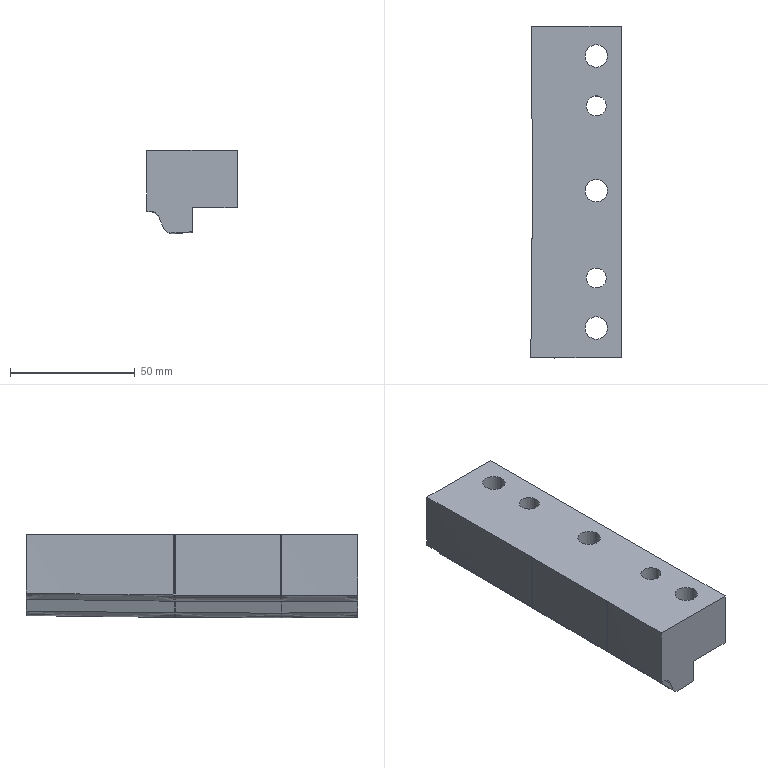Part | STEP file | 811_id1618_x_t | 1 solid | 45 faces | box 36.277 x 133 x 33.411 mm | volume 115856 mm3 | spline 24 | plane 11 | cylinder 10 | commonest cylinder face diameters 9 x3 14 x3 8 x2 10 x2